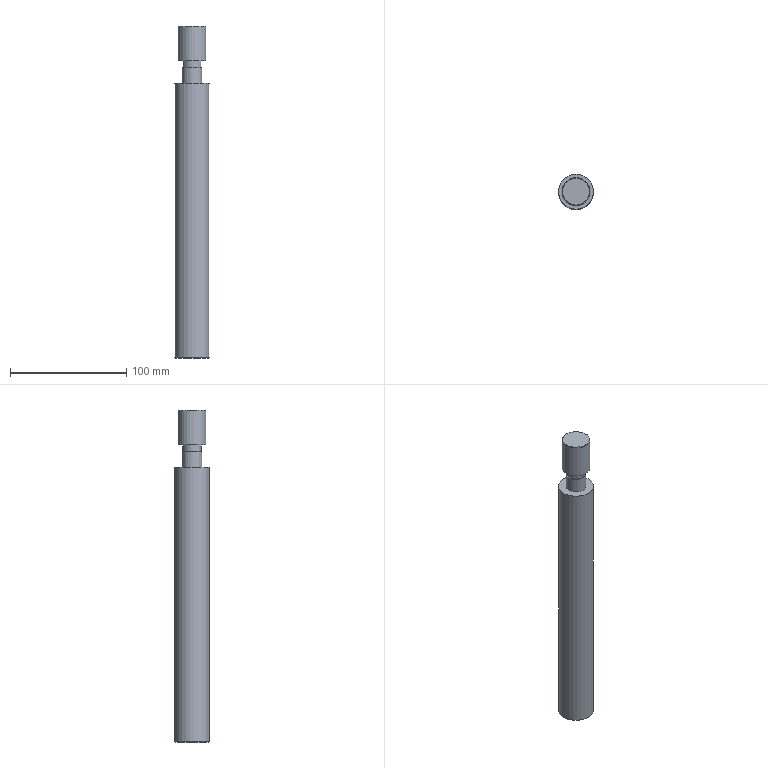Part | NX | features solid 2 | 1 solid | 11 faces | box 30 x 30 x 285 mm | volume 184526 mm3 | plane 5 | cylinder 4 | cone 2 | commonest cylinder face diameters 16 x1 17 x1 24 x1 30 x1
STEP:
#1=CARTESIAN_POINT('',(255.,-95.,-269.5));
#2=VERTEX_POINT('',#1);
#3=CARTESIAN_POINT('',(255.,-80.,-269.5));
#4=DIRECTION('',(0.,0.,-1.));
#5=DIRECTION('',(0.,-1.,0.));
#6=AXIS2_PLACEMENT_3D('',#3,#4,#5);
#7=CIRCLE('',#6,15.);
#8=EDGE_CURVE('',#2,#2,#7,.F.);
#9=ORIENTED_EDGE('',*,*,#8,.T.);
#10=EDGE_LOOP('',(#9));
#11=FACE_BOUND('',#10,.T.);
#12=CARTESIAN_POINT('',(255.,-95.,-34.));
#13=VERTEX_POINT('',#12);
#14=CARTESIAN_POINT('',(255.,-80.,-34.));
#15=DIRECTION('',(0.,0.,-1.));
#16=DIRECTION('',(0.,-1.,0.));
#17=AXIS2_PLACEMENT_3D('',#14,#15,#16);
#18=CIRCLE('',#17,15.);
#19=EDGE_CURVE('',#13,#13,#18,.F.);
#20=ORIENTED_EDGE('',*,*,#19,.F.);
#21=EDGE_LOOP('',(#20));
#22=FACE_BOUND('',#21,.T.);
#23=CARTESIAN_POINT('',(255.,-80.,-270.));
#24=DIRECTION('',(0.,0.,1.));
#25=DIRECTION('',(0.,-1.,0.));
#26=AXIS2_PLACEMENT_3D('',#23,#24,#25);
#27=CYLINDRICAL_SURFACE('',#26,15.);
#28=ADVANCED_FACE('',(#11,#22),#27,.T.);
#29=CARTESIAN_POINT('',(255.,-88.5,-34.));
#30=VERTEX_POINT('',#29);
#31=CARTESIAN_POINT('',(255.,-80.,-34.));
#32=DIRECTION('',(0.,0.,1.));
#33=DIRECTION('',(0.,-1.,0.));
#34=AXIS2_PLACEMENT_3D('',#31,#32,#33);
#35=CIRCLE('',#34,8.5);
#36=EDGE_CURVE('',#30,#30,#35,.T.);
#37=ORIENTED_EDGE('',*,*,#36,.F.);
#38=EDGE_LOOP('',(#37));
#39=FACE_BOUND('',#38,.T.);
#40=ORIENTED_EDGE('',*,*,#19,.T.);
#41=EDGE_LOOP('',(#40));
#42=FACE_BOUND('',#41,.T.);
#43=CARTESIAN_POINT('',(255.,-80.,-34.));
#44=DIRECTION('',(0.,0.,-1.));
#45=DIRECTION('',(0.,1.,0.));
#46=AXIS2_PLACEMENT_3D('',#43,#44,#45);
#47=PLANE('',#46);
#48=ADVANCED_FACE('',(#39,#42),#47,.F.);
#49=CARTESIAN_POINT('',(255.,-94.5,-270.));
#50=VERTEX_POINT('',#49);
#51=CARTESIAN_POINT('',(255.,-80.,-270.));
#52=DIRECTION('',(0.,0.,-1.));
#53=DIRECTION('',(0.,-1.,0.));
#54=AXIS2_PLACEMENT_3D('',#51,#52,#53);
#55=CIRCLE('',#54,14.5);
#56=EDGE_CURVE('',#50,#50,#55,.T.);
#57=ORIENTED_EDGE('',*,*,#56,.T.);
#58=EDGE_LOOP('',(#57));
#59=FACE_BOUND('',#58,.T.);
#60=CARTESIAN_POINT('',(255.,-80.,-270.));
#61=DIRECTION('',(0.,0.,-1.));
#62=DIRECTION('',(0.,1.,0.));
#63=AXIS2_PLACEMENT_3D('',#60,#61,#62);
#64=PLANE('',#63);
#65=ADVANCED_FACE('',(#59),#64,.T.);
#66=CARTESIAN_POINT('',(255.,-71.5,-21.));
#67=VERTEX_POINT('',#66);
#68=CARTESIAN_POINT('',(255.,-80.,-21.));
#69=DIRECTION('',(0.,0.,1.));
#70=DIRECTION('',(0.,1.,0.));
#71=AXIS2_PLACEMENT_3D('',#68,#69,#70);
#72=CIRCLE('',#71,8.5);
#73=EDGE_CURVE('',#67,#67,#72,.T.);
#74=ORIENTED_EDGE('',*,*,#73,.F.);
#75=EDGE_LOOP('',(#74));
#76=FACE_BOUND('',#75,.T.);
#77=ORIENTED_EDGE('',*,*,#36,.T.);
#78=EDGE_LOOP('',(#77));
#79=FACE_BOUND('',#78,.T.);
#80=CARTESIAN_POINT('',(255.,-80.,-34.));
#81=DIRECTION('',(0.,0.,1.));
#82=DIRECTION('',(0.,-1.,0.));
#83=AXIS2_PLACEMENT_3D('',#80,#81,#82);
#84=CYLINDRICAL_SURFACE('',#83,8.5);
#85=ADVANCED_FACE('',(#76,#79),#84,.T.);
#86=CARTESIAN_POINT('',(255.,-88.,-21.));
#87=VERTEX_POINT('',#86);
#88=CARTESIAN_POINT('',(255.,-80.,-21.));
#89=DIRECTION('',(0.,0.,1.));
#90=DIRECTION('',(0.,-1.,0.));
#91=AXIS2_PLACEMENT_3D('',#88,#89,#90);
#92=CIRCLE('',#91,8.);
#93=EDGE_CURVE('',#87,#87,#92,.T.);
#94=ORIENTED_EDGE('',*,*,#93,.F.);
#95=EDGE_LOOP('',(#94));
#96=FACE_BOUND('',#95,.T.);
#97=ORIENTED_EDGE('',*,*,#73,.T.);
#98=EDGE_LOOP('',(#97));
#99=FACE_BOUND('',#98,.T.);
#100=CARTESIAN_POINT('',(255.,-80.,-21.));
#101=DIRECTION('',(0.,0.,-1.));
#102=DIRECTION('',(0.,1.,0.));
#103=AXIS2_PLACEMENT_3D('',#100,#101,#102);
#104=PLANE('',#103);
#105=ADVANCED_FACE('',(#96,#99),#104,.F.);
#106=ORIENTED_EDGE('',*,*,#93,.T.);
#107=EDGE_LOOP('',(#106));
#108=FACE_BOUND('',#107,.T.);
#109=CARTESIAN_POINT('',(255.,-88.,-15.));
#110=VERTEX_POINT('',#109);
#111=CARTESIAN_POINT('',(255.,-80.,-15.));
#112=DIRECTION('',(0.,0.,1.));
#113=DIRECTION('',(0.,-1.,0.));
#114=AXIS2_PLACEMENT_3D('',#111,#112,#113);
#115=CIRCLE('',#114,8.);
#116=EDGE_CURVE('',#110,#110,#115,.T.);
#117=ORIENTED_EDGE('',*,*,#116,.F.);
#118=EDGE_LOOP('',(#117));
#119=FACE_BOUND('',#118,.T.);
#120=CARTESIAN_POINT('',(255.,-80.,-21.));
#121=DIRECTION('',(0.,0.,1.));
#122=DIRECTION('',(0.,-1.,0.));
#123=AXIS2_PLACEMENT_3D('',#120,#121,#122);
#124=CYLINDRICAL_SURFACE('',#123,8.);
#125=ADVANCED_FACE('',(#108,#119),#124,.T.);
#126=CARTESIAN_POINT('',(255.,-91.5,15.));
#127=VERTEX_POINT('',#126);
#128=CARTESIAN_POINT('',(255.,-80.,15.));
#129=DIRECTION('',(0.,0.,-1.));
#130=DIRECTION('',(0.,-1.,0.));
#131=AXIS2_PLACEMENT_3D('',#128,#129,#130);
#132=CIRCLE('',#131,11.5);
#133=EDGE_CURVE('',#127,#127,#132,.F.);
#134=ORIENTED_EDGE('',*,*,#133,.T.);
#135=EDGE_LOOP('',(#134));
#136=FACE_BOUND('',#135,.T.);
#137=CARTESIAN_POINT('',(255.,-80.,15.));
#138=DIRECTION('',(0.,0.,-1.));
#139=DIRECTION('',(0.,1.,0.));
#140=AXIS2_PLACEMENT_3D('',#137,#138,#139);
#141=PLANE('',#140);
#142=ADVANCED_FACE('',(#136),#141,.F.);
#143=CARTESIAN_POINT('',(255.,-92.,14.5));
#144=VERTEX_POINT('',#143);
#145=CARTESIAN_POINT('',(255.,-80.,14.5));
#146=DIRECTION('',(0.,0.,-1.));
#147=DIRECTION('',(0.,-1.,0.));
#148=AXIS2_PLACEMENT_3D('',#145,#146,#147);
#149=CIRCLE('',#148,12.);
#150=EDGE_CURVE('',#144,#144,#149,.T.);
#151=ORIENTED_EDGE('',*,*,#150,.T.);
#152=EDGE_LOOP('',(#151));
#153=FACE_BOUND('',#152,.T.);
#154=CARTESIAN_POINT('',(255.,-92.,-15.));
#155=VERTEX_POINT('',#154);
#156=CARTESIAN_POINT('',(255.,-80.,-15.));
#157=DIRECTION('',(0.,0.,-1.));
#158=DIRECTION('',(0.,-1.,0.));
#159=AXIS2_PLACEMENT_3D('',#156,#157,#158);
#160=CIRCLE('',#159,12.);
#161=EDGE_CURVE('',#155,#155,#160,.F.);
#162=ORIENTED_EDGE('',*,*,#161,.T.);
#163=EDGE_LOOP('',(#162));
#164=FACE_BOUND('',#163,.T.);
#165=CARTESIAN_POINT('',(255.,-80.,-270.));
#166=DIRECTION('',(0.,0.,1.));
#167=DIRECTION('',(0.,-1.,0.));
#168=AXIS2_PLACEMENT_3D('',#165,#166,#167);
#169=CYLINDRICAL_SURFACE('',#168,12.);
#170=ADVANCED_FACE('',(#153,#164),#169,.T.);
#171=ORIENTED_EDGE('',*,*,#161,.F.);
#172=EDGE_LOOP('',(#171));
#173=FACE_BOUND('',#172,.T.);
#174=ORIENTED_EDGE('',*,*,#116,.T.);
#175=EDGE_LOOP('',(#174));
#176=FACE_BOUND('',#175,.T.);
#177=CARTESIAN_POINT('',(255.,-80.,-15.));
#178=DIRECTION('',(0.,0.,-1.));
#179=DIRECTION('',(0.,1.,0.));
#180=AXIS2_PLACEMENT_3D('',#177,#178,#179);
#181=PLANE('',#180);
#182=ADVANCED_FACE('',(#173,#176),#181,.T.);
#183=ORIENTED_EDGE('',*,*,#56,.F.);
#184=EDGE_LOOP('',(#183));
#185=FACE_BOUND('',#184,.T.);
#186=ORIENTED_EDGE('',*,*,#8,.F.);
#187=EDGE_LOOP('',(#186));
#188=FACE_BOUND('',#187,.T.);
#189=CARTESIAN_POINT('',(255.,-80.,-269.5));
#190=DIRECTION('',(0.,0.,1.));
#191=DIRECTION('',(0.,1.,0.));
#192=AXIS2_PLACEMENT_3D('',#189,#190,#191);
#193=CONICAL_SURFACE('',#192,15.,0.7854);
#194=ADVANCED_FACE('',(#185,#188),#193,.T.);
#195=ORIENTED_EDGE('',*,*,#150,.F.);
#196=EDGE_LOOP('',(#195));
#197=FACE_BOUND('',#196,.T.);
#198=ORIENTED_EDGE('',*,*,#133,.F.);
#199=EDGE_LOOP('',(#198));
#200=FACE_BOUND('',#199,.T.);
#201=CARTESIAN_POINT('',(255.,-80.,15.));
#202=DIRECTION('',(0.,0.,-1.));
#203=DIRECTION('',(0.,-1.,0.));
#204=AXIS2_PLACEMENT_3D('',#201,#202,#203);
#205=CONICAL_SURFACE('',#204,11.5,0.7854);
#206=ADVANCED_FACE('',(#197,#200),#205,.T.);
#207=CLOSED_SHELL('',(#28,#48,#65,#85,#105,#125,#142,#170,#182,#194,#206));
#208=MANIFOLD_SOLID_BREP('',#207);
#209=(LENGTH_UNIT()NAMED_UNIT(*)SI_UNIT(.MILLI.,.METRE.));
#210=UNCERTAINTY_MEASURE_WITH_UNIT(LENGTH_MEASURE(0.00001),#209,'','');
#211=(NAMED_UNIT(*)PLANE_ANGLE_UNIT()SI_UNIT($,.RADIAN.));
#212=(NAMED_UNIT(*)SI_UNIT($,.STERADIAN.)SOLID_ANGLE_UNIT());
#213=(GEOMETRIC_REPRESENTATION_CONTEXT(3)GLOBAL_UNCERTAINTY_ASSIGNED_CONTEXT((#210))GLOBAL_UNIT_ASSIGNED_CONTEXT((#209,#211,#212))REPRESENTATION_CONTEXT('',''));
#214=ADVANCED_BREP_SHAPE_REPRESENTATION('',(#208),#213);